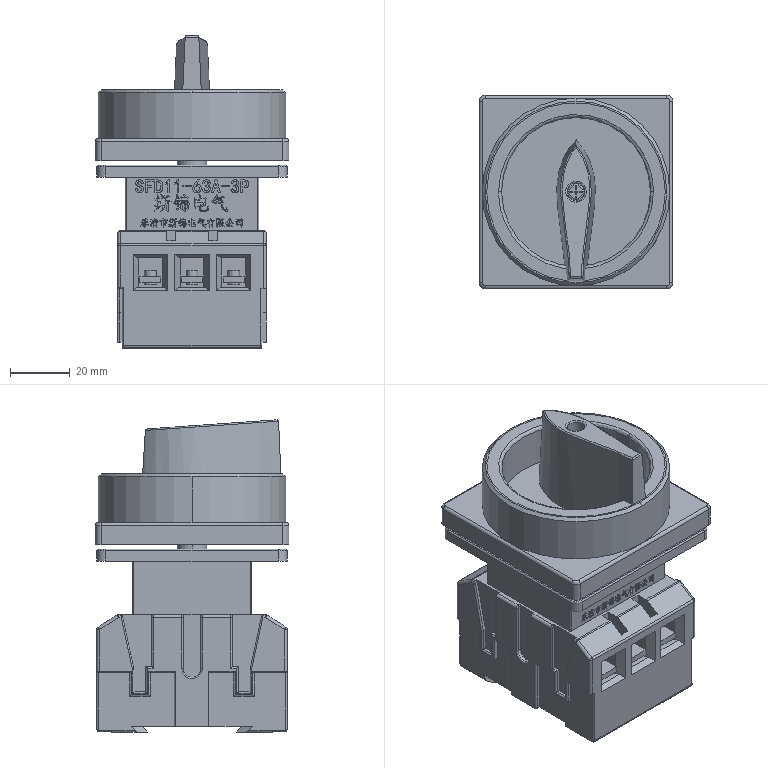Part | SolidWorks | features BaseBody 9 | 9 solids | 1699 faces | box 65 x 65 x 104.965 mm | volume 219842 mm3 | plane 1014 | spline 482 | cylinder 185 | cone 18 | commonest cylinder face diameters 1 x52 4 x40 2 x30 7.5 x12 8 x12 6 x9